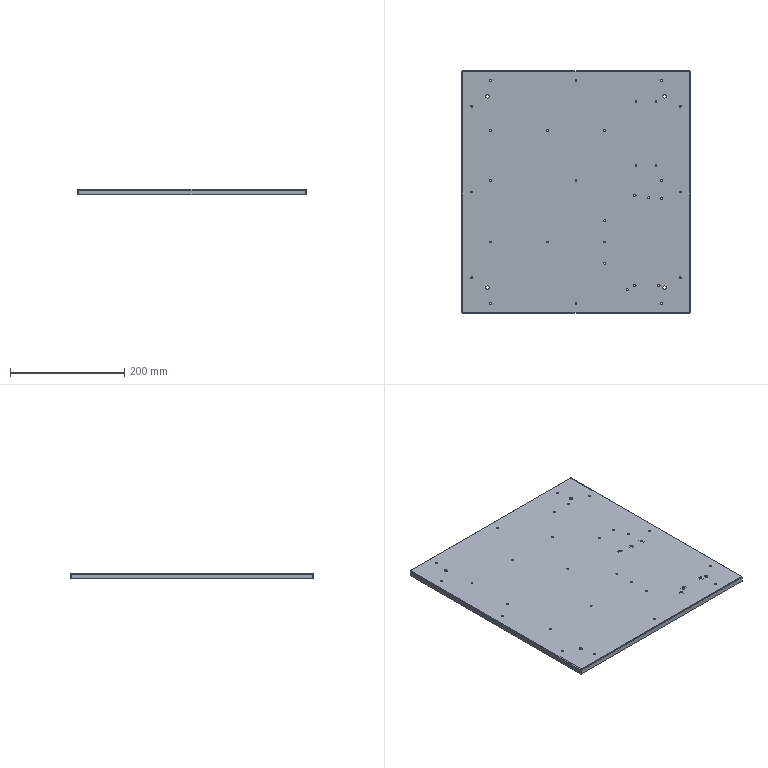Part | STEP file | 1 solid | 130 faces | box 400 x 425 x 10 mm | volume 275109 mm3 | cylinder 94 | plane 28 | spline 8 | commonest cylinder face diameters 3.3 x58 4.2 x8 6 x8 10 x8 0.2 x4 3.2 x4